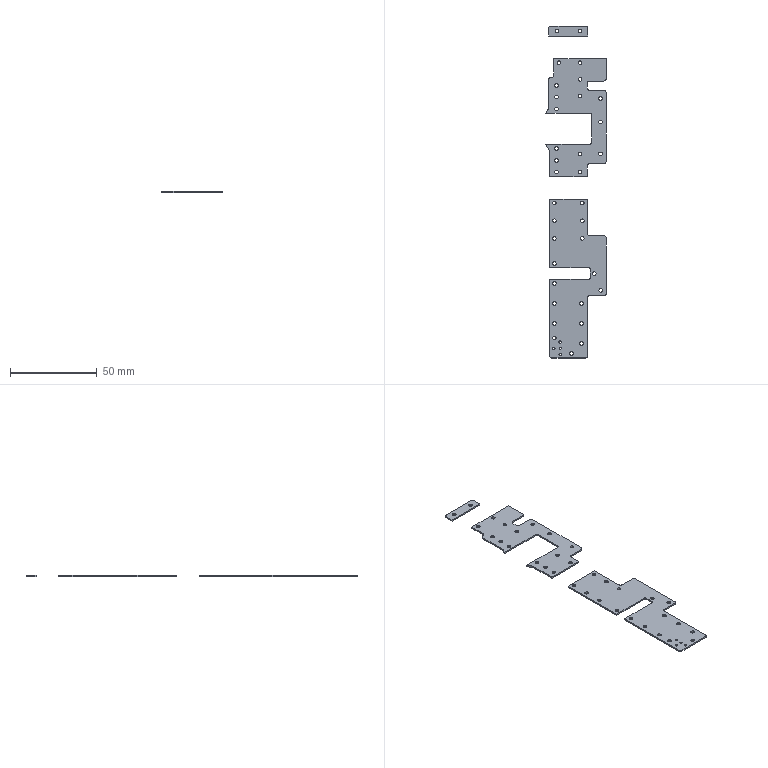Part | STEP file | Final stage amplifier 00 | 3 solids | 104 faces | box 34.739 x 191 x 0.832 mm | volume 3190 mm3 | cylinder 64 | plane 40 | commonest cylinder face diameters 2.1 x34 2.54 x19 1.4 x3 6.132 x3 0.9 x2 1.2 x1